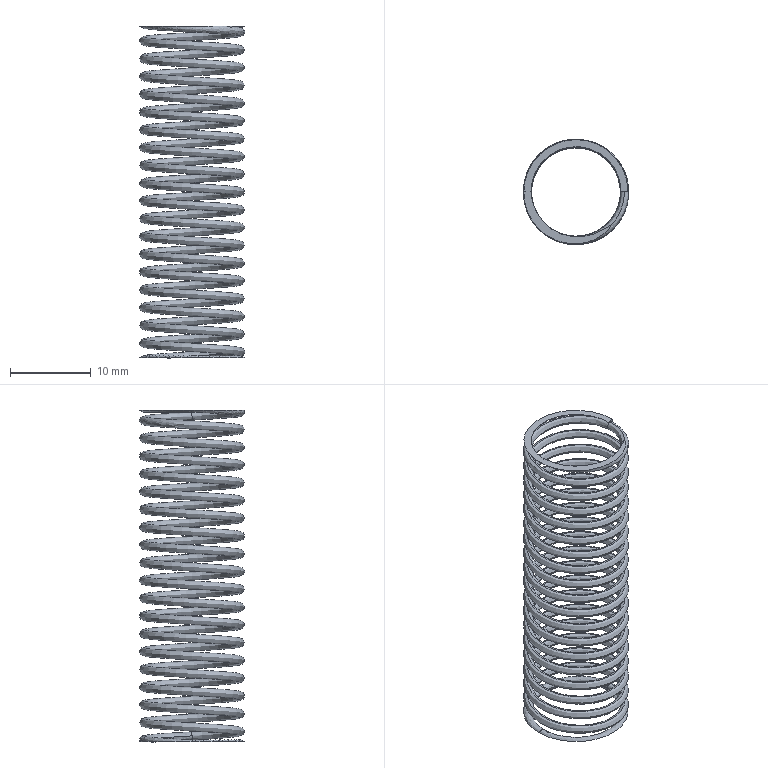Part | SolidWorks | features Helix 3, Cut 2, CompositeCurve 1, Sweep 1 | 1 solid | 13 faces | box 13 x 13 x 41 mm | volume 559.424 mm3 | spline 9 | plane 4